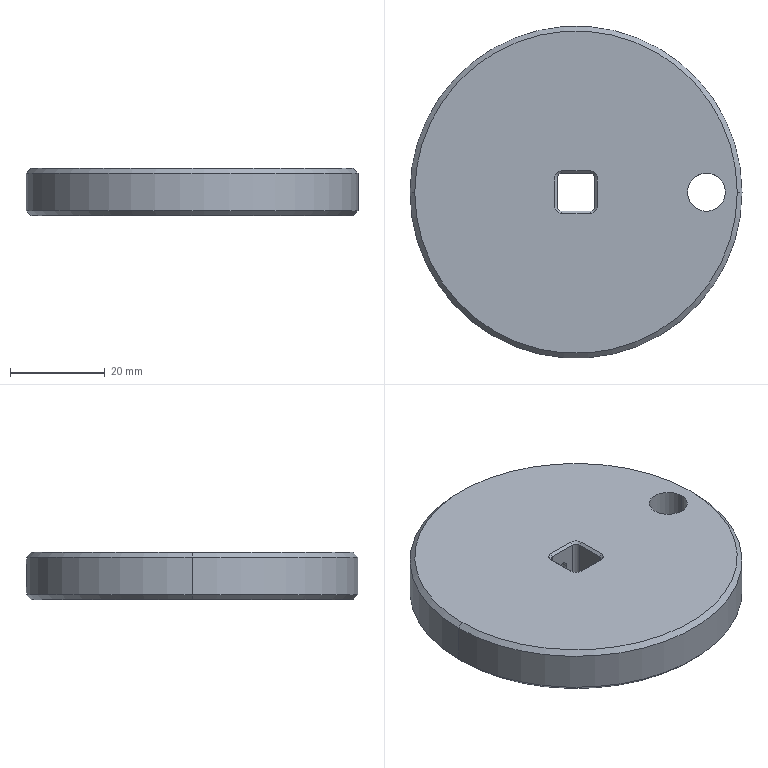Part | SolidWorks | features ICE 4, Chamfer 2, 3DProfileFeature 1, Cut 1, Extrusion 1, Fillet 1, HoleWzd 1 | 1 solid | 39 faces | box 70 x 70 x 10 mm | volume 36483 mm3 | plane 15 | cylinder 12 | cone 12 | commonest cylinder face diameters 2 x4 2.5 x2 6 x2 8 x2 70 x2
STEP:
#1=CARTESIAN_POINT('',(0.,4.,3.75));
#2=VERTEX_POINT('',#1);
#3=CARTESIAN_POINT('',(0.,4.,6.25));
#4=VERTEX_POINT('',#3);
#5=CARTESIAN_POINT('',(0.,4.,5.));
#6=DIRECTION('',(0.,1.,0.));
#7=DIRECTION('',(0.,0.,1.));
#8=AXIS2_PLACEMENT_3D('',#5,#6,#7);
#9=CIRCLE('',#8,1.25);
#10=EDGE_CURVE('',#2,#4,#9,.T.);
#11=ORIENTED_EDGE('',*,*,#10,.F.);
#12=CARTESIAN_POINT('',(0.,14.,3.75));
#13=VERTEX_POINT('',#12);
#14=CARTESIAN_POINT('',(0.,14.,3.75));
#15=DIRECTION('',(0.,1.,0.));
#16=VECTOR('',#15,1000.);
#17=LINE('',#14,#16);
#18=EDGE_CURVE('',#2,#13,#17,.T.);
#19=ORIENTED_EDGE('',*,*,#18,.T.);
#20=CARTESIAN_POINT('',(0.,14.,6.25));
#21=VERTEX_POINT('',#20);
#22=CARTESIAN_POINT('',(0.,14.,5.));
#23=DIRECTION('',(0.,1.,0.));
#24=DIRECTION('',(0.,0.,1.));
#25=AXIS2_PLACEMENT_3D('',#22,#23,#24);
#26=CIRCLE('',#25,1.25);
#27=EDGE_CURVE('',#13,#21,#26,.T.);
#28=ORIENTED_EDGE('',*,*,#27,.T.);
#29=CARTESIAN_POINT('',(0.,14.,6.25));
#30=DIRECTION('',(0.,1.,0.));
#31=VECTOR('',#30,1000.);
#32=LINE('',#29,#31);
#33=EDGE_CURVE('',#4,#21,#32,.T.);
#34=ORIENTED_EDGE('',*,*,#33,.F.);
#35=EDGE_LOOP('',(#11,#19,#28,#34));
#36=FACE_OUTER_BOUND('',#35,.T.);
#37=CARTESIAN_POINT('',(0.,14.,5.));
#38=DIRECTION('',(0.,1.,0.));
#39=DIRECTION('',(0.,0.,1.));
#40=AXIS2_PLACEMENT_3D('',#37,#38,#39);
#41=CYLINDRICAL_SURFACE('',#40,1.25);
#42=ADVANCED_FACE('',(#36),#41,.F.);
#43=CARTESIAN_POINT('',(0.,35.,2.));
#44=VERTEX_POINT('',#43);
#45=CARTESIAN_POINT('',(0.,35.,8.));
#46=VERTEX_POINT('',#45);
#47=CARTESIAN_POINT('',(0.,35.,2.));
#48=CARTESIAN_POINT('',(-0.1983,35.,2.));
#49=CARTESIAN_POINT('',(-0.3933,34.998,2.019));
#50=CARTESIAN_POINT('',(-0.7769,34.992,2.096));
#51=CARTESIAN_POINT('',(-0.9675,34.987,2.153));
#52=CARTESIAN_POINT('',(-1.331,34.975,2.304));
#53=CARTESIAN_POINT('',(-1.503,34.968,2.396));
#54=CARTESIAN_POINT('',(-1.829,34.953,2.614));
#55=CARTESIAN_POINT('',(-1.983,34.944,2.741));
#56=CARTESIAN_POINT('',(-2.26,34.927,3.017));
#57=CARTESIAN_POINT('',(-2.384,34.919,3.168));
#58=CARTESIAN_POINT('',(-2.603,34.903,3.496));
#59=CARTESIAN_POINT('',(-2.697,34.896,3.671));
#60=CARTESIAN_POINT('',(-2.846,34.884,4.032));
#61=CARTESIAN_POINT('',(-2.904,34.879,4.221));
#62=CARTESIAN_POINT('',(-2.981,34.873,4.608));
#63=CARTESIAN_POINT('',(-3.,34.871,4.803));
#64=CARTESIAN_POINT('',(-3.,34.871,5.195));
#65=CARTESIAN_POINT('',(-2.981,34.873,5.394));
#66=CARTESIAN_POINT('',(-2.904,34.879,5.778));
#67=CARTESIAN_POINT('',(-2.847,34.884,5.965));
#68=CARTESIAN_POINT('',(-2.697,34.896,6.329));
#69=CARTESIAN_POINT('',(-2.603,34.903,6.504));
#70=CARTESIAN_POINT('',(-2.386,34.919,6.829));
#71=CARTESIAN_POINT('',(-2.262,34.927,6.981));
#72=CARTESIAN_POINT('',(-1.982,34.944,7.261));
#73=CARTESIAN_POINT('',(-1.83,34.952,7.385));
#74=CARTESIAN_POINT('',(-1.505,34.968,7.602));
#75=CARTESIAN_POINT('',(-1.33,34.975,7.696));
#76=CARTESIAN_POINT('',(-0.9664,34.987,7.847));
#77=CARTESIAN_POINT('',(-0.7794,34.992,7.904));
#78=CARTESIAN_POINT('',(-0.3948,34.998,7.98));
#79=CARTESIAN_POINT('',(-0.1958,35.,8.));
#80=CARTESIAN_POINT('',(0.,35.,8.));
#81=B_SPLINE_CURVE_WITH_KNOTS('',3,(#47,#48,#49,#50,#51,#52,#53,#54,#55,#56,#57,#58,#59,#60,#61,#62,#63,#64,#65,#66,#67,#68,#69,#70,#71,#72,#73,#74,#75,#76,#77,#78,#79,#80),.UNSPECIFIED.,.F.,.F.,(4,2,2,2,2,2,2,2,2,2,2,2,2,2,2,2,4),(0.,0.0005865,0.001173,0.001759,0.002346,0.002932,0.003519,0.004105,0.004692,0.005278,0.005865,0.006451,0.007038,0.007624,0.008211,0.008797,0.009384),.UNSPECIFIED.);
#82=EDGE_CURVE('',#44,#46,#81,.T.);
#83=ORIENTED_EDGE('',*,*,#82,.T.);
#84=CARTESIAN_POINT('',(0.,14.,8.));
#85=VERTEX_POINT('',#84);
#86=CARTESIAN_POINT('',(0.,35.027,8.));
#87=DIRECTION('',(0.,-1.,0.));
#88=VECTOR('',#87,1000.);
#89=LINE('',#86,#88);
#90=EDGE_CURVE('',#46,#85,#89,.T.);
#91=ORIENTED_EDGE('',*,*,#90,.T.);
#92=CARTESIAN_POINT('',(0.,14.,2.));
#93=VERTEX_POINT('',#92);
#94=CARTESIAN_POINT('',(0.,14.,5.));
#95=DIRECTION('',(0.,1.,0.));
#96=DIRECTION('',(0.,0.,1.));
#97=AXIS2_PLACEMENT_3D('',#94,#95,#96);
#98=CIRCLE('',#97,3.);
#99=EDGE_CURVE('',#93,#85,#98,.T.);
#100=ORIENTED_EDGE('',*,*,#99,.F.);
#101=CARTESIAN_POINT('',(0.,35.027,2.));
#102=DIRECTION('',(0.,-1.,0.));
#103=VECTOR('',#102,1000.);
#104=LINE('',#101,#103);
#105=EDGE_CURVE('',#44,#93,#104,.T.);
#106=ORIENTED_EDGE('',*,*,#105,.F.);
#107=EDGE_LOOP('',(#83,#91,#100,#106));
#108=FACE_OUTER_BOUND('',#107,.T.);
#109=CARTESIAN_POINT('',(0.,35.027,5.));
#110=DIRECTION('',(0.,-1.,0.));
#111=DIRECTION('',(0.,0.,-1.));
#112=AXIS2_PLACEMENT_3D('',#109,#110,#111);
#113=CYLINDRICAL_SURFACE('',#112,3.);
#114=ADVANCED_FACE('',(#108),#113,.F.);
#115=CARTESIAN_POINT('',(23.5,0.,0.));
#116=VERTEX_POINT('',#115);
#117=CARTESIAN_POINT('',(31.5,0.,0.));
#118=VERTEX_POINT('',#117);
#119=CARTESIAN_POINT('',(27.5,0.,0.));
#120=DIRECTION('',(0.,0.,1.));
#121=DIRECTION('',(1.,0.,0.));
#122=AXIS2_PLACEMENT_3D('',#119,#120,#121);
#123=CIRCLE('',#122,4.);
#124=EDGE_CURVE('',#116,#118,#123,.T.);
#125=ORIENTED_EDGE('',*,*,#124,.F.);
#126=CARTESIAN_POINT('',(23.5,0.,10.));
#127=VERTEX_POINT('',#126);
#128=CARTESIAN_POINT('',(23.5,0.,-19.));
#129=DIRECTION('',(0.,0.,1.));
#130=VECTOR('',#129,1000.);
#131=LINE('',#128,#130);
#132=EDGE_CURVE('',#116,#127,#131,.T.);
#133=ORIENTED_EDGE('',*,*,#132,.T.);
#134=CARTESIAN_POINT('',(31.5,0.,10.));
#135=VERTEX_POINT('',#134);
#136=CARTESIAN_POINT('',(27.5,0.,10.));
#137=DIRECTION('',(0.,0.,1.));
#138=DIRECTION('',(1.,0.,0.));
#139=AXIS2_PLACEMENT_3D('',#136,#137,#138);
#140=CIRCLE('',#139,4.);
#141=EDGE_CURVE('',#127,#135,#140,.T.);
#142=ORIENTED_EDGE('',*,*,#141,.T.);
#143=CARTESIAN_POINT('',(31.5,0.,-19.));
#144=DIRECTION('',(0.,0.,1.));
#145=VECTOR('',#144,1000.);
#146=LINE('',#143,#145);
#147=EDGE_CURVE('',#118,#135,#146,.T.);
#148=ORIENTED_EDGE('',*,*,#147,.F.);
#149=EDGE_LOOP('',(#125,#133,#142,#148));
#150=FACE_OUTER_BOUND('',#149,.T.);
#151=CARTESIAN_POINT('',(27.5,0.,-19.));
#152=DIRECTION('',(0.,0.,1.));
#153=DIRECTION('',(1.,0.,0.));
#154=AXIS2_PLACEMENT_3D('',#151,#152,#153);
#155=CYLINDRICAL_SURFACE('',#154,4.);
#156=ADVANCED_FACE('',(#150),#155,.F.);
#157=CARTESIAN_POINT('',(34.,0.,10.));
#158=VERTEX_POINT('',#157);
#159=CARTESIAN_POINT('',(-34.,0.,10.));
#160=VERTEX_POINT('',#159);
#161=CARTESIAN_POINT('',(0.,0.,10.));
#162=DIRECTION('',(0.,0.,1.));
#163=DIRECTION('',(1.,0.,0.));
#164=AXIS2_PLACEMENT_3D('',#161,#162,#163);
#165=CIRCLE('',#164,34.);
#166=EDGE_CURVE('',#158,#160,#165,.T.);
#167=ORIENTED_EDGE('',*,*,#166,.F.);
#168=CARTESIAN_POINT('',(35.,0.,9.));
#169=VERTEX_POINT('',#168);
#170=CARTESIAN_POINT('',(34.,0.,10.));
#171=DIRECTION('',(0.7071,0.,-0.7071));
#172=VECTOR('',#171,1000.);
#173=LINE('',#170,#172);
#174=EDGE_CURVE('',#158,#169,#173,.T.);
#175=ORIENTED_EDGE('',*,*,#174,.T.);
#176=CARTESIAN_POINT('',(-35.,0.,9.));
#177=VERTEX_POINT('',#176);
#178=CARTESIAN_POINT('',(0.,0.,9.));
#179=DIRECTION('',(0.,0.,-1.));
#180=DIRECTION('',(1.,0.,0.));
#181=AXIS2_PLACEMENT_3D('',#178,#179,#180);
#182=CIRCLE('',#181,35.);
#183=EDGE_CURVE('',#177,#169,#182,.T.);
#184=ORIENTED_EDGE('',*,*,#183,.F.);
#185=CARTESIAN_POINT('',(-34.,0.,10.));
#186=DIRECTION('',(-0.7071,0.,-0.7071));
#187=VECTOR('',#186,1000.);
#188=LINE('',#185,#187);
#189=EDGE_CURVE('',#160,#177,#188,.T.);
#190=ORIENTED_EDGE('',*,*,#189,.F.);
#191=EDGE_LOOP('',(#167,#175,#184,#190));
#192=FACE_OUTER_BOUND('',#191,.T.);
#193=CARTESIAN_POINT('',(0.,0.,10.));
#194=DIRECTION('',(0.,0.,-1.));
#195=DIRECTION('',(-1.,0.,0.));
#196=AXIS2_PLACEMENT_3D('',#193,#194,#195);
#197=CONICAL_SURFACE('',#196,34.,0.7854);
#198=ADVANCED_FACE('',(#192),#197,.T.);
#199=CARTESIAN_POINT('',(-34.,0.,0.));
#200=VERTEX_POINT('',#199);
#201=CARTESIAN_POINT('',(34.,0.,0.));
#202=VERTEX_POINT('',#201);
#203=CARTESIAN_POINT('',(0.,0.,0.));
#204=DIRECTION('',(0.,0.,-1.));
#205=DIRECTION('',(1.,0.,0.));
#206=AXIS2_PLACEMENT_3D('',#203,#204,#205);
#207=CIRCLE('',#206,34.);
#208=EDGE_CURVE('',#200,#202,#207,.T.);
#209=ORIENTED_EDGE('',*,*,#208,.F.);
#210=CARTESIAN_POINT('',(-35.,0.,1.));
#211=VERTEX_POINT('',#210);
#212=CARTESIAN_POINT('',(-35.,0.,1.));
#213=DIRECTION('',(-0.7071,0.,0.7071));
#214=VECTOR('',#213,1000.);
#215=LINE('',#212,#214);
#216=EDGE_CURVE('',#200,#211,#215,.T.);
#217=ORIENTED_EDGE('',*,*,#216,.T.);
#218=CARTESIAN_POINT('',(35.,0.,1.));
#219=VERTEX_POINT('',#218);
#220=CARTESIAN_POINT('',(0.,0.,1.));
#221=DIRECTION('',(0.,0.,1.));
#222=DIRECTION('',(1.,0.,0.));
#223=AXIS2_PLACEMENT_3D('',#220,#221,#222);
#224=CIRCLE('',#223,35.);
#225=EDGE_CURVE('',#219,#211,#224,.T.);
#226=ORIENTED_EDGE('',*,*,#225,.F.);
#227=CARTESIAN_POINT('',(35.,0.,1.));
#228=DIRECTION('',(0.7071,0.,0.7071));
#229=VECTOR('',#228,1000.);
#230=LINE('',#227,#229);
#231=EDGE_CURVE('',#202,#219,#230,.T.);
#232=ORIENTED_EDGE('',*,*,#231,.F.);
#233=EDGE_LOOP('',(#209,#217,#226,#232));
#234=FACE_OUTER_BOUND('',#233,.T.);
#235=CARTESIAN_POINT('',(0.,0.,1.));
#236=DIRECTION('',(0.,0.,1.));
#237=DIRECTION('',(1.,0.,0.));
#238=AXIS2_PLACEMENT_3D('',#235,#236,#237);
#239=CONICAL_SURFACE('',#238,35.,0.7854);
#240=ADVANCED_FACE('',(#234),#239,.T.);
#241=ORIENTED_EDGE('',*,*,#82,.F.);
#242=CARTESIAN_POINT('',(0.,35.,8.));
#243=CARTESIAN_POINT('',(0.1958,35.,8.));
#244=CARTESIAN_POINT('',(0.3904,34.998,7.981));
#245=CARTESIAN_POINT('',(0.7774,34.992,7.904));
#246=CARTESIAN_POINT('',(0.9669,34.987,7.847));
#247=CARTESIAN_POINT('',(1.328,34.975,7.697));
#248=CARTESIAN_POINT('',(1.502,34.968,7.604));
#249=CARTESIAN_POINT('',(1.83,34.952,7.385));
#250=CARTESIAN_POINT('',(1.981,34.944,7.261));
#251=CARTESIAN_POINT('',(2.258,34.927,6.985));
#252=CARTESIAN_POINT('',(2.385,34.919,6.83));
#253=CARTESIAN_POINT('',(2.603,34.903,6.504));
#254=CARTESIAN_POINT('',(2.695,34.896,6.332));
#255=CARTESIAN_POINT('',(2.846,34.884,5.969));
#256=CARTESIAN_POINT('',(2.904,34.879,5.779));
#257=CARTESIAN_POINT('',(2.98,34.873,5.395));
#258=CARTESIAN_POINT('',(3.,34.871,5.2));
#259=CARTESIAN_POINT('',(3.,34.871,4.804));
#260=CARTESIAN_POINT('',(2.981,34.873,4.609));
#261=CARTESIAN_POINT('',(2.905,34.879,4.225));
#262=CARTESIAN_POINT('',(2.847,34.884,4.035));
#263=CARTESIAN_POINT('',(2.697,34.896,3.671));
#264=CARTESIAN_POINT('',(2.605,34.903,3.499));
#265=CARTESIAN_POINT('',(2.388,34.919,3.173));
#266=CARTESIAN_POINT('',(2.261,34.927,3.019));
#267=CARTESIAN_POINT('',(1.985,34.944,2.742));
#268=CARTESIAN_POINT('',(1.834,34.952,2.618));
#269=CARTESIAN_POINT('',(1.506,34.968,2.398));
#270=CARTESIAN_POINT('',(1.332,34.975,2.305));
#271=CARTESIAN_POINT('',(0.7905,34.993,2.08));
#272=CARTESIAN_POINT('',(0.3965,35.,2.));
#273=CARTESIAN_POINT('',(0.,35.,2.));
#274=B_SPLINE_CURVE_WITH_KNOTS('',3,(#242,#243,#244,#245,#246,#247,#248,#249,#250,#251,#252,#253,#254,#255,#256,#257,#258,#259,#260,#261,#262,#263,#264,#265,#266,#267,#268,#269,#270,#271,#272,#273),.UNSPECIFIED.,.F.,.F.,(4,2,2,2,2,2,2,2,2,2,2,2,2,2,2,4),(0.009384,0.00997,0.01056,0.01114,0.01173,0.01232,0.0129,0.01349,0.01407,0.01466,0.01525,0.01583,0.01642,0.01701,0.01759,0.01877),.UNSPECIFIED.);
#275=EDGE_CURVE('',#46,#44,#274,.T.);
#276=ORIENTED_EDGE('',*,*,#275,.F.);
#277=EDGE_LOOP('',(#241,#276));
#278=FACE_BOUND('',#277,.T.);
#279=ORIENTED_EDGE('',*,*,#183,.T.);
#280=CARTESIAN_POINT('',(35.,0.,10.));
#281=DIRECTION('',(0.,0.,-1.));
#282=VECTOR('',#281,1000.);
#283=LINE('',#280,#282);
#284=EDGE_CURVE('',#169,#219,#283,.T.);
#285=ORIENTED_EDGE('',*,*,#284,.T.);
#286=ORIENTED_EDGE('',*,*,#225,.T.);
#287=CARTESIAN_POINT('',(-35.,0.,10.));
#288=DIRECTION('',(0.,0.,-1.));
#289=VECTOR('',#288,1000.);
#290=LINE('',#287,#289);
#291=EDGE_CURVE('',#177,#211,#290,.T.);
#292=ORIENTED_EDGE('',*,*,#291,.F.);
#293=EDGE_LOOP('',(#279,#285,#286,#292));
#294=FACE_OUTER_BOUND('',#293,.T.);
#295=CARTESIAN_POINT('',(0.,0.,10.));
#296=DIRECTION('',(0.,0.,-1.));
#297=DIRECTION('',(-1.,0.,0.));
#298=AXIS2_PLACEMENT_3D('',#295,#296,#297);
#299=CYLINDRICAL_SURFACE('',#298,35.);
#300=ADVANCED_FACE('',(#278,#294),#299,.T.);
#301=ORIENTED_EDGE('',*,*,#284,.F.);
#302=CARTESIAN_POINT('',(0.,0.,9.));
#303=DIRECTION('',(0.,0.,-1.));
#304=DIRECTION('',(1.,0.,0.));
#305=AXIS2_PLACEMENT_3D('',#302,#303,#304);
#306=CIRCLE('',#305,35.);
#307=EDGE_CURVE('',#169,#177,#306,.T.);
#308=ORIENTED_EDGE('',*,*,#307,.T.);
#309=ORIENTED_EDGE('',*,*,#291,.T.);
#310=CARTESIAN_POINT('',(0.,0.,1.));
#311=DIRECTION('',(0.,0.,1.));
#312=DIRECTION('',(1.,0.,0.));
#313=AXIS2_PLACEMENT_3D('',#310,#311,#312);
#314=CIRCLE('',#313,35.);
#315=EDGE_CURVE('',#211,#219,#314,.T.);
#316=ORIENTED_EDGE('',*,*,#315,.T.);
#317=EDGE_LOOP('',(#301,#308,#309,#316));
#318=FACE_OUTER_BOUND('',#317,.T.);
#319=CARTESIAN_POINT('',(0.,0.,10.));
#320=DIRECTION('',(0.,0.,-1.));
#321=DIRECTION('',(-1.,0.,0.));
#322=AXIS2_PLACEMENT_3D('',#319,#320,#321);
#323=CYLINDRICAL_SURFACE('',#322,35.);
#324=ADVANCED_FACE('',(#318),#323,.T.);
#325=CARTESIAN_POINT('',(3.,4.5,10.));
#326=VERTEX_POINT('',#325);
#327=CARTESIAN_POINT('',(4.5,3.,10.));
#328=VERTEX_POINT('',#327);
#329=CARTESIAN_POINT('',(3.,3.,10.));
#330=DIRECTION('',(0.,0.,-1.));
#331=DIRECTION('',(1.,0.,0.));
#332=AXIS2_PLACEMENT_3D('',#329,#330,#331);
#333=CIRCLE('',#332,1.5);
#334=EDGE_CURVE('',#326,#328,#333,.T.);
#335=ORIENTED_EDGE('',*,*,#334,.T.);
#336=CARTESIAN_POINT('',(4.5,-3.,10.));
#337=VERTEX_POINT('',#336);
#338=CARTESIAN_POINT('',(4.5,-3.,10.));
#339=DIRECTION('',(0.,-1.,0.));
#340=VECTOR('',#339,1000.);
#341=LINE('',#338,#340);
#342=EDGE_CURVE('',#328,#337,#341,.T.);
#343=ORIENTED_EDGE('',*,*,#342,.T.);
#344=CARTESIAN_POINT('',(3.,-4.5,10.));
#345=VERTEX_POINT('',#344);
#346=CARTESIAN_POINT('',(3.,-3.,10.));
#347=DIRECTION('',(0.,0.,-1.));
#348=DIRECTION('',(1.,0.,0.));
#349=AXIS2_PLACEMENT_3D('',#346,#347,#348);
#350=CIRCLE('',#349,1.5);
#351=EDGE_CURVE('',#337,#345,#350,.T.);
#352=ORIENTED_EDGE('',*,*,#351,.T.);
#353=CARTESIAN_POINT('',(-3.,-4.5,10.));
#354=VERTEX_POINT('',#353);
#355=CARTESIAN_POINT('',(-3.,-4.5,10.));
#356=DIRECTION('',(-1.,0.,0.));
#357=VECTOR('',#356,1000.);
#358=LINE('',#355,#357);
#359=EDGE_CURVE('',#345,#354,#358,.T.);
#360=ORIENTED_EDGE('',*,*,#359,.T.);
#361=CARTESIAN_POINT('',(-4.5,-3.,10.));
#362=VERTEX_POINT('',#361);
#363=CARTESIAN_POINT('',(-3.,-3.,10.));
#364=DIRECTION('',(0.,0.,-1.));
#365=DIRECTION('',(1.,0.,0.));
#366=AXIS2_PLACEMENT_3D('',#363,#364,#365);
#367=CIRCLE('',#366,1.5);
#368=EDGE_CURVE('',#354,#362,#367,.T.);
#369=ORIENTED_EDGE('',*,*,#368,.T.);
#370=CARTESIAN_POINT('',(-4.5,3.,10.));
#371=VERTEX_POINT('',#370);
#372=CARTESIAN_POINT('',(-4.5,3.,10.));
#373=DIRECTION('',(0.,1.,0.));
#374=VECTOR('',#373,1000.);
#375=LINE('',#372,#374);
#376=EDGE_CURVE('',#362,#371,#375,.T.);
#377=ORIENTED_EDGE('',*,*,#376,.T.);
#378=CARTESIAN_POINT('',(-3.,4.5,10.));
#379=VERTEX_POINT('',#378);
#380=CARTESIAN_POINT('',(-3.,3.,10.));
#381=DIRECTION('',(0.,0.,-1.));
#382=DIRECTION('',(1.,0.,0.));
#383=AXIS2_PLACEMENT_3D('',#380,#381,#382);
#384=CIRCLE('',#383,1.5);
#385=EDGE_CURVE('',#371,#379,#384,.T.);
#386=ORIENTED_EDGE('',*,*,#385,.T.);
#387=CARTESIAN_POINT('',(3.,4.5,10.));
#388=DIRECTION('',(1.,0.,0.));
#389=VECTOR('',#388,1000.);
#390=LINE('',#387,#389);
#391=EDGE_CURVE('',#379,#326,#390,.T.);
#392=ORIENTED_EDGE('',*,*,#391,.T.);
#393=EDGE_LOOP('',(#335,#343,#352,#360,#369,#377,#386,#392));
#394=FACE_BOUND('',#393,.T.);
#395=CARTESIAN_POINT('',(27.5,0.,10.));
#396=DIRECTION('',(0.,0.,1.));
#397=DIRECTION('',(1.,0.,0.));
#398=AXIS2_PLACEMENT_3D('',#395,#396,#397);
#399=CIRCLE('',#398,4.);
#400=EDGE_CURVE('',#135,#127,#399,.T.);
#401=ORIENTED_EDGE('',*,*,#400,.F.);
#402=ORIENTED_EDGE('',*,*,#141,.F.);
#403=EDGE_LOOP('',(#401,#402));
#404=FACE_BOUND('',#403,.T.);
#405=CARTESIAN_POINT('',(0.,0.,10.));
#406=DIRECTION('',(0.,0.,1.));
#407=DIRECTION('',(1.,0.,0.));
#408=AXIS2_PLACEMENT_3D('',#405,#406,#407);
#409=CIRCLE('',#408,34.);
#410=EDGE_CURVE('',#160,#158,#409,.T.);
#411=ORIENTED_EDGE('',*,*,#410,.T.);
#412=ORIENTED_EDGE('',*,*,#166,.T.);
#413=EDGE_LOOP('',(#411,#412));
#414=FACE_OUTER_BOUND('',#413,.T.);
#415=CARTESIAN_POINT('',(0.,0.,10.));
#416=DIRECTION('',(0.,0.,1.));
#417=DIRECTION('',(1.,0.,0.));
#418=AXIS2_PLACEMENT_3D('',#415,#416,#417);
#419=PLANE('',#418);
#420=ADVANCED_FACE('',(#394,#404,#414),#419,.T.);
#421=CARTESIAN_POINT('',(-4.5,-3.,0.));
#422=VERTEX_POINT('',#421);
#423=CARTESIAN_POINT('',(-3.,-4.5,0.));
#424=VERTEX_POINT('',#423);
#425=CARTESIAN_POINT('',(-3.,-3.,0.));
#426=DIRECTION('',(0.,0.,1.));
#427=DIRECTION('',(1.,0.,0.));
#428=AXIS2_PLACEMENT_3D('',#425,#426,#427);
#429=CIRCLE('',#428,1.5);
#430=EDGE_CURVE('',#422,#424,#429,.T.);
#431=ORIENTED_EDGE('',*,*,#430,.T.);
#432=CARTESIAN_POINT('',(3.,-4.5,0.));
#433=VERTEX_POINT('',#432);
#434=CARTESIAN_POINT('',(0.,-4.5,0.));
#435=DIRECTION('',(1.,0.,0.));
#436=VECTOR('',#435,1000.);
#437=LINE('',#434,#436);
#438=EDGE_CURVE('',#424,#433,#437,.T.);
#439=ORIENTED_EDGE('',*,*,#438,.T.);
#440=CARTESIAN_POINT('',(4.5,-3.,0.));
#441=VERTEX_POINT('',#440);
#442=CARTESIAN_POINT('',(3.,-3.,0.));
#443=DIRECTION('',(0.,0.,1.));
#444=DIRECTION('',(1.,0.,0.));
#445=AXIS2_PLACEMENT_3D('',#442,#443,#444);
#446=CIRCLE('',#445,1.5);
#447=EDGE_CURVE('',#433,#441,#446,.T.);
#448=ORIENTED_EDGE('',*,*,#447,.T.);
#449=CARTESIAN_POINT('',(4.5,3.,0.));
#450=VERTEX_POINT('',#449);
#451=CARTESIAN_POINT('',(4.5,0.,0.));
#452=DIRECTION('',(0.,1.,0.));
#453=VECTOR('',#452,1000.);
#454=LINE('',#451,#453);
#455=EDGE_CURVE('',#441,#450,#454,.T.);
#456=ORIENTED_EDGE('',*,*,#455,.T.);
#457=CARTESIAN_POINT('',(3.,4.5,0.));
#458=VERTEX_POINT('',#457);
#459=CARTESIAN_POINT('',(3.,3.,0.));
#460=DIRECTION('',(0.,0.,1.));
#461=DIRECTION('',(1.,0.,0.));
#462=AXIS2_PLACEMENT_3D('',#459,#460,#461);
#463=CIRCLE('',#462,1.5);
#464=EDGE_CURVE('',#450,#458,#463,.T.);
#465=ORIENTED_EDGE('',*,*,#464,.T.);
#466=CARTESIAN_POINT('',(-3.,4.5,0.));
#467=VERTEX_POINT('',#466);
#468=CARTESIAN_POINT('',(0.,4.5,0.));
#469=DIRECTION('',(-1.,0.,0.));
#470=VECTOR('',#469,1000.);
#471=LINE('',#468,#470);
#472=EDGE_CURVE('',#458,#467,#471,.T.);
#473=ORIENTED_EDGE('',*,*,#472,.T.);
#474=CARTESIAN_POINT('',(-4.5,3.,0.));
#475=VERTEX_POINT('',#474);
#476=CARTESIAN_POINT('',(-3.,3.,0.));
#477=DIRECTION('',(0.,0.,1.));
#478=DIRECTION('',(1.,0.,0.));
#479=AXIS2_PLACEMENT_3D('',#476,#477,#478);
#480=CIRCLE('',#479,1.5);
#481=EDGE_CURVE('',#467,#475,#480,.T.);
#482=ORIENTED_EDGE('',*,*,#481,.T.);
#483=CARTESIAN_POINT('',(-4.5,0.,0.));
#484=DIRECTION('',(0.,-1.,0.));
#485=VECTOR('',#484,1000.);
#486=LINE('',#483,#485);
#487=EDGE_CURVE('',#475,#422,#486,.T.);
#488=ORIENTED_EDGE('',*,*,#487,.T.);
#489=EDGE_LOOP('',(#431,#439,#448,#456,#465,#473,#482,#488));
#490=FACE_BOUND('',#489,.T.);
#491=CARTESIAN_POINT('',(27.5,0.,0.));
#492=DIRECTION('',(0.,0.,1.));
#493=DIRECTION('',(1.,0.,0.));
#494=AXIS2_PLACEMENT_3D('',#491,#492,#493);
#495=CIRCLE('',#494,4.);
#496=EDGE_CURVE('',#118,#116,#495,.T.);
#497=ORIENTED_EDGE('',*,*,#496,.T.);
#498=ORIENTED_EDGE('',*,*,#124,.T.);
#499=EDGE_LOOP('',(#497,#498));
#500=FACE_BOUND('',#499,.T.);
#501=CARTESIAN_POINT('',(0.,0.,0.));
#502=DIRECTION('',(0.,0.,-1.));
#503=DIRECTION('',(1.,0.,0.));
#504=AXIS2_PLACEMENT_3D('',#501,#502,#503);
#505=CIRCLE('',#504,34.);
#506=EDGE_CURVE('',#202,#200,#505,.T.);
#507=ORIENTED_EDGE('',*,*,#506,.T.);
#508=ORIENTED_EDGE('',*,*,#208,.T.);
#509=EDGE_LOOP('',(#507,#508));
#510=FACE_OUTER_BOUND('',#509,.T.);
#511=CARTESIAN_POINT('',(0.,0.,0.));
#512=DIRECTION('',(0.,0.,1.));
#513=DIRECTION('',(1.,0.,0.));
#514=AXIS2_PLACEMENT_3D('',#511,#512,#513);
#515=PLANE('',#514);
#516=ADVANCED_FACE('',(#490,#500,#510),#515,.F.);
#517=ORIENTED_EDGE('',*,*,#216,.F.);
#518=ORIENTED_EDGE('',*,*,#506,.F.);
#519=ORIENTED_EDGE('',*,*,#231,.T.);
#520=ORIENTED_EDGE('',*,*,#315,.F.);
#521=EDGE_LOOP('',(#517,#518,#519,#520));
#522=FACE_OUTER_BOUND('',#521,.T.);
#523=CARTESIAN_POINT('',(0.,0.,1.));
#524=DIRECTION('',(0.,0.,1.));
#525=DIRECTION('',(1.,0.,0.));
#526=AXIS2_PLACEMENT_3D('',#523,#524,#525);
#527=CONICAL_SURFACE('',#526,35.,0.7854);
#528=ADVANCED_FACE('',(#522),#527,.T.);
#529=ORIENTED_EDGE('',*,*,#174,.F.);
#530=ORIENTED_EDGE('',*,*,#410,.F.);
#531=ORIENTED_EDGE('',*,*,#189,.T.);
#532=ORIENTED_EDGE('',*,*,#307,.F.);
#533=EDGE_LOOP('',(#529,#530,#531,#532));
#534=FACE_OUTER_BOUND('',#533,.T.);
#535=CARTESIAN_POINT('',(0.,0.,10.));
#536=DIRECTION('',(0.,0.,-1.));
#537=DIRECTION('',(-1.,0.,0.));
#538=AXIS2_PLACEMENT_3D('',#535,#536,#537);
#539=CONICAL_SURFACE('',#538,34.,0.7854);
#540=ADVANCED_FACE('',(#534),#539,.T.);
#541=ORIENTED_EDGE('',*,*,#132,.F.);
#542=ORIENTED_EDGE('',*,*,#496,.F.);
#543=ORIENTED_EDGE('',*,*,#147,.T.);
#544=ORIENTED_EDGE('',*,*,#400,.T.);
#545=EDGE_LOOP('',(#541,#542,#543,#544));
#546=FACE_OUTER_BOUND('',#545,.T.);
#547=CARTESIAN_POINT('',(27.5,0.,-19.));
#548=DIRECTION('',(0.,0.,1.));
#549=DIRECTION('',(1.,0.,0.));
#550=AXIS2_PLACEMENT_3D('',#547,#548,#549);
#551=CYLINDRICAL_SURFACE('',#550,4.);
#552=ADVANCED_FACE('',(#546),#551,.F.);
#553=CARTESIAN_POINT('',(4.,3.,9.5));
#554=VERTEX_POINT('',#553);
#555=CARTESIAN_POINT('',(4.,3.,0.5));
#556=VERTEX_POINT('',#555);
#557=CARTESIAN_POINT('',(4.,3.,0.));
#558=DIRECTION('',(0.,0.,-1.));
#559=VECTOR('',#558,1000.);
#560=LINE('',#557,#559);
#561=EDGE_CURVE('',#554,#556,#560,.T.);
#562=ORIENTED_EDGE('',*,*,#561,.T.);
#563=CARTESIAN_POINT('',(4.,-3.,0.5));
#564=VERTEX_POINT('',#563);
#565=CARTESIAN_POINT('',(4.,4.,0.5));
#566=DIRECTION('',(0.,-1.,0.));
#567=VECTOR('',#566,1000.);
#568=LINE('',#565,#567);
#569=EDGE_CURVE('',#556,#564,#568,.T.);
#570=ORIENTED_EDGE('',*,*,#569,.T.);
#571=CARTESIAN_POINT('',(4.,-3.,9.5));
#572=VERTEX_POINT('',#571);
#573=CARTESIAN_POINT('',(4.,-3.,10.));
#574=DIRECTION('',(0.,0.,1.));
#575=VECTOR('',#574,1000.);
#576=LINE('',#573,#575);
#577=EDGE_CURVE('',#564,#572,#576,.T.);
#578=ORIENTED_EDGE('',*,*,#577,.T.);
#579=CARTESIAN_POINT('',(4.,3.,9.5));
#580=DIRECTION('',(0.,1.,0.));
#581=VECTOR('',#580,1000.);
#582=LINE('',#579,#581);
#583=EDGE_CURVE('',#572,#554,#582,.T.);
#584=ORIENTED_EDGE('',*,*,#583,.T.);
#585=EDGE_LOOP('',(#562,#570,#578,#584));
#586=FACE_OUTER_BOUND('',#585,.T.);
#587=CARTESIAN_POINT('',(4.,4.,0.));
#588=DIRECTION('',(1.,0.,0.));
#589=DIRECTION('',(0.,1.,0.));
#590=AXIS2_PLACEMENT_3D('',#587,#588,#589);
#591=PLANE('',#590);
#592=ADVANCED_FACE('',(#586),#591,.F.);
#593=CARTESIAN_POINT('',(3.,-4.,9.5));
#594=VERTEX_POINT('',#593);
#595=CARTESIAN_POINT('',(3.,-4.,0.5));
#596=VERTEX_POINT('',#595);
#597=CARTESIAN_POINT('',(3.,-4.,0.));
#598=DIRECTION('',(0.,0.,-1.));
#599=VECTOR('',#598,1000.);
#600=LINE('',#597,#599);
#601=EDGE_CURVE('',#594,#596,#600,.T.);
#602=ORIENTED_EDGE('',*,*,#601,.T.);
#603=CARTESIAN_POINT('',(-3.,-4.,0.5));
#604=VERTEX_POINT('',#603);
#605=CARTESIAN_POINT('',(-4.,-4.,0.5));
#606=DIRECTION('',(-1.,0.,0.));
#607=VECTOR('',#606,1000.);
#608=LINE('',#605,#607);
#609=EDGE_CURVE('',#596,#604,#608,.T.);
#610=ORIENTED_EDGE('',*,*,#609,.T.);
#611=CARTESIAN_POINT('',(-3.,-4.,9.5));
#612=VERTEX_POINT('',#611);
#613=CARTESIAN_POINT('',(-3.,-4.,10.));
#614=DIRECTION('',(0.,0.,1.));
#615=VECTOR('',#614,1000.);
#616=LINE('',#613,#615);
#617=EDGE_CURVE('',#604,#612,#616,.T.);
#618=ORIENTED_EDGE('',*,*,#617,.T.);
#619=CARTESIAN_POINT('',(3.,-4.,9.5));
#620=DIRECTION('',(1.,0.,0.));
#621=VECTOR('',#620,1000.);
#622=LINE('',#619,#621);
#623=EDGE_CURVE('',#612,#594,#622,.T.);
#624=ORIENTED_EDGE('',*,*,#623,.T.);
#625=EDGE_LOOP('',(#602,#610,#618,#624));
#626=FACE_OUTER_BOUND('',#625,.T.);
#627=CARTESIAN_POINT('',(-4.,-4.,0.));
#628=DIRECTION('',(0.,-1.,0.));
#629=DIRECTION('',(0.,0.,-1.));
#630=AXIS2_PLACEMENT_3D('',#627,#628,#629);
#631=PLANE('',#630);
#632=ADVANCED_FACE('',(#626),#631,.F.);
#633=CARTESIAN_POINT('',(-4.,-3.,9.5));
#634=VERTEX_POINT('',#633);
#635=CARTESIAN_POINT('',(-4.,-3.,0.5));
#636=VERTEX_POINT('',#635);
#637=CARTESIAN_POINT('',(-4.,-3.,0.));
#638=DIRECTION('',(0.,0.,-1.));
#639=VECTOR('',#638,1000.);
#640=LINE('',#637,#639);
#641=EDGE_CURVE('',#634,#636,#640,.T.);
#642=ORIENTED_EDGE('',*,*,#641,.T.);
#643=CARTESIAN_POINT('',(-4.,3.,0.5));
#644=VERTEX_POINT('',#643);
#645=CARTESIAN_POINT('',(-4.,4.,0.5));
#646=DIRECTION('',(0.,1.,0.));
#647=VECTOR('',#646,1000.);
#648=LINE('',#645,#647);
#649=EDGE_CURVE('',#636,#644,#648,.T.);
#650=ORIENTED_EDGE('',*,*,#649,.T.);
#651=CARTESIAN_POINT('',(-4.,3.,9.5));
#652=VERTEX_POINT('',#651);
#653=CARTESIAN_POINT('',(-4.,3.,10.));
#654=DIRECTION('',(0.,0.,1.));
#655=VECTOR('',#654,1000.);
#656=LINE('',#653,#655);
#657=EDGE_CURVE('',#644,#652,#656,.T.);
#658=ORIENTED_EDGE('',*,*,#657,.T.);
#659=CARTESIAN_POINT('',(-4.,-3.,9.5));
#660=DIRECTION('',(0.,-1.,0.));
#661=VECTOR('',#660,1000.);
#662=LINE('',#659,#661);
#663=EDGE_CURVE('',#652,#634,#662,.T.);
#664=ORIENTED_EDGE('',*,*,#663,.T.);
#665=EDGE_LOOP('',(#642,#650,#658,#664));
#666=FACE_OUTER_BOUND('',#665,.T.);
#667=CARTESIAN_POINT('',(-4.,4.,0.));
#668=DIRECTION('',(-1.,0.,0.));
#669=DIRECTION('',(0.,-1.,0.));
#670=AXIS2_PLACEMENT_3D('',#667,#668,#669);
#671=PLANE('',#670);
#672=ADVANCED_FACE('',(#666),#671,.F.);
#673=CARTESIAN_POINT('',(0.,4.,5.));
#674=DIRECTION('',(0.,1.,0.));
#675=DIRECTION('',(0.,0.,1.));
#676=AXIS2_PLACEMENT_3D('',#673,#674,#675);
#677=CIRCLE('',#676,1.25);
#678=EDGE_CURVE('',#4,#2,#677,.T.);
#679=ORIENTED_EDGE('',*,*,#678,.T.);
#680=ORIENTED_EDGE('',*,*,#10,.T.);
#681=EDGE_LOOP('',(#679,#680));
#682=FACE_BOUND('',#681,.T.);
#683=CARTESIAN_POINT('',(-3.,4.,9.5));
#684=VERTEX_POINT('',#683);
#685=CARTESIAN_POINT('',(-3.,4.,0.5));
#686=VERTEX_POINT('',#685);
#687=CARTESIAN_POINT('',(-3.,4.,0.));
#688=DIRECTION('',(0.,0.,-1.));
#689=VECTOR('',#688,1000.);
#690=LINE('',#687,#689);
#691=EDGE_CURVE('',#684,#686,#690,.T.);
#692=ORIENTED_EDGE('',*,*,#691,.T.);
#693=CARTESIAN_POINT('',(3.,4.,0.5));
#694=VERTEX_POINT('',#693);
#695=CARTESIAN_POINT('',(-4.,4.,0.5));
#696=DIRECTION('',(1.,0.,0.));
#697=VECTOR('',#696,1000.);
#698=LINE('',#695,#697);
#699=EDGE_CURVE('',#686,#694,#698,.T.);
#700=ORIENTED_EDGE('',*,*,#699,.T.);
#701=CARTESIAN_POINT('',(3.,4.,9.5));
#702=VERTEX_POINT('',#701);
#703=CARTESIAN_POINT('',(3.,4.,10.));
#704=DIRECTION('',(0.,0.,1.));
#705=VECTOR('',#704,1000.);
#706=LINE('',#703,#705);
#707=EDGE_CURVE('',#694,#702,#706,.T.);
#708=ORIENTED_EDGE('',*,*,#707,.T.);
#709=CARTESIAN_POINT('',(-3.,4.,9.5));
#710=DIRECTION('',(-1.,0.,0.));
#711=VECTOR('',#710,1000.);
#712=LINE('',#709,#711);
#713=EDGE_CURVE('',#702,#684,#712,.T.);
#714=ORIENTED_EDGE('',*,*,#713,.T.);
#715=EDGE_LOOP('',(#692,#700,#708,#714));
#716=FACE_OUTER_BOUND('',#715,.T.);
#717=CARTESIAN_POINT('',(-4.,4.,0.));
#718=DIRECTION('',(0.,1.,0.));
#719=DIRECTION('',(0.,0.,1.));
#720=AXIS2_PLACEMENT_3D('',#717,#718,#719);
#721=PLANE('',#720);
#722=ADVANCED_FACE('',(#682,#716),#721,.F.);
#723=ORIENTED_EDGE('',*,*,#617,.F.);
#724=CARTESIAN_POINT('',(-3.,-3.,0.5));
#725=DIRECTION('',(0.,0.,-1.));
#726=DIRECTION('',(1.,0.,0.));
#727=AXIS2_PLACEMENT_3D('',#724,#725,#726);
#728=CIRCLE('',#727,1.);
#729=EDGE_CURVE('',#604,#636,#728,.T.);
#730=ORIENTED_EDGE('',*,*,#729,.T.);
#731=ORIENTED_EDGE('',*,*,#641,.F.);
#732=CARTESIAN_POINT('',(-3.,-3.,9.5));
#733=DIRECTION('',(0.,0.,1.));
#734=DIRECTION('',(1.,0.,0.));
#735=AXIS2_PLACEMENT_3D('',#732,#733,#734);
#736=CIRCLE('',#735,1.);
#737=EDGE_CURVE('',#634,#612,#736,.T.);
#738=ORIENTED_EDGE('',*,*,#737,.T.);
#739=EDGE_LOOP('',(#723,#730,#731,#738));
#740=FACE_OUTER_BOUND('',#739,.T.);
#741=CARTESIAN_POINT('',(-3.,-3.,0.));
#742=DIRECTION('',(0.,0.,-1.));
#743=DIRECTION('',(-1.,0.,0.));
#744=AXIS2_PLACEMENT_3D('',#741,#742,#743);
#745=CYLINDRICAL_SURFACE('',#744,1.);
#746=ADVANCED_FACE('',(#740),#745,.F.);
#747=ORIENTED_EDGE('',*,*,#577,.F.);
#748=CARTESIAN_POINT('',(3.,-3.,0.5));
#749=DIRECTION('',(0.,0.,-1.));
#750=DIRECTION('',(1.,0.,0.));
#751=AXIS2_PLACEMENT_3D('',#748,#749,#750);
#752=CIRCLE('',#751,1.);
#753=EDGE_CURVE('',#564,#596,#752,.T.);
#754=ORIENTED_EDGE('',*,*,#753,.T.);
#755=ORIENTED_EDGE('',*,*,#601,.F.);
#756=CARTESIAN_POINT('',(3.,-3.,9.5));
#757=DIRECTION('',(0.,0.,1.));
#758=DIRECTION('',(1.,0.,0.));
#759=AXIS2_PLACEMENT_3D('',#756,#757,#758);
#760=CIRCLE('',#759,1.);
#761=EDGE_CURVE('',#594,#572,#760,.T.);
#762=ORIENTED_EDGE('',*,*,#761,.T.);
#763=EDGE_LOOP('',(#747,#754,#755,#762));
#764=FACE_OUTER_BOUND('',#763,.T.);
#765=CARTESIAN_POINT('',(3.,-3.,0.));
#766=DIRECTION('',(0.,0.,-1.));
#767=DIRECTION('',(-1.,0.,0.));
#768=AXIS2_PLACEMENT_3D('',#765,#766,#767);
#769=CYLINDRICAL_SURFACE('',#768,1.);
#770=ADVANCED_FACE('',(#764),#769,.F.);
#771=ORIENTED_EDGE('',*,*,#707,.F.);
#772=CARTESIAN_POINT('',(3.,3.,0.5));
#773=DIRECTION('',(0.,0.,-1.));
#774=DIRECTION('',(1.,0.,0.));
#775=AXIS2_PLACEMENT_3D('',#772,#773,#774);
#776=CIRCLE('',#775,1.);
#777=EDGE_CURVE('',#694,#556,#776,.T.);
#778=ORIENTED_EDGE('',*,*,#777,.T.);
#779=ORIENTED_EDGE('',*,*,#561,.F.);
#780=CARTESIAN_POINT('',(3.,3.,9.5));
#781=DIRECTION('',(0.,0.,1.));
#782=DIRECTION('',(1.,0.,0.));
#783=AXIS2_PLACEMENT_3D('',#780,#781,#782);
#784=CIRCLE('',#783,1.);
#785=EDGE_CURVE('',#554,#702,#784,.T.);
#786=ORIENTED_EDGE('',*,*,#785,.T.);
#787=EDGE_LOOP('',(#771,#778,#779,#786));
#788=FACE_OUTER_BOUND('',#787,.T.);
#789=CARTESIAN_POINT('',(3.,3.,0.));
#790=DIRECTION('',(0.,0.,-1.));
#791=DIRECTION('',(-1.,0.,0.));
#792=AXIS2_PLACEMENT_3D('',#789,#790,#791);
#793=CYLINDRICAL_SURFACE('',#792,1.);
#794=ADVANCED_FACE('',(#788),#793,.F.);
#795=ORIENTED_EDGE('',*,*,#657,.F.);
#796=CARTESIAN_POINT('',(-3.,3.,0.5));
#797=DIRECTION('',(0.,0.,-1.));
#798=DIRECTION('',(1.,0.,0.));
#799=AXIS2_PLACEMENT_3D('',#796,#797,#798);
#800=CIRCLE('',#799,1.);
#801=EDGE_CURVE('',#644,#686,#800,.T.);
#802=ORIENTED_EDGE('',*,*,#801,.T.);
#803=ORIENTED_EDGE('',*,*,#691,.F.);
#804=CARTESIAN_POINT('',(-3.,3.,9.5));
#805=DIRECTION('',(0.,0.,1.));
#806=DIRECTION('',(1.,0.,0.));
#807=AXIS2_PLACEMENT_3D('',#804,#805,#806);
#808=CIRCLE('',#807,1.);
#809=EDGE_CURVE('',#684,#652,#808,.T.);
#810=ORIENTED_EDGE('',*,*,#809,.T.);
#811=EDGE_LOOP('',(#795,#802,#803,#810));
#812=FACE_OUTER_BOUND('',#811,.T.);
#813=CARTESIAN_POINT('',(-3.,3.,0.));
#814=DIRECTION('',(0.,0.,-1.));
#815=DIRECTION('',(-1.,0.,0.));
#816=AXIS2_PLACEMENT_3D('',#813,#814,#815);
#817=CYLINDRICAL_SURFACE('',#816,1.);
#818=ADVANCED_FACE('',(#812),#817,.F.);
#819=ORIENTED_EDGE('',*,*,#90,.F.);
#820=ORIENTED_EDGE('',*,*,#275,.T.);
#821=ORIENTED_EDGE('',*,*,#105,.T.);
#822=CARTESIAN_POINT('',(0.,14.,5.));
#823=DIRECTION('',(0.,1.,0.));
#824=DIRECTION('',(0.,0.,1.));
#825=AXIS2_PLACEMENT_3D('',#822,#823,#824);
#826=CIRCLE('',#825,3.);
#827=EDGE_CURVE('',#85,#93,#826,.T.);
#828=ORIENTED_EDGE('',*,*,#827,.F.);
#829=EDGE_LOOP('',(#819,#820,#821,#828));
#830=FACE_OUTER_BOUND('',#829,.T.);
#831=CARTESIAN_POINT('',(0.,35.027,5.));
#832=DIRECTION('',(0.,-1.,0.));
#833=DIRECTION('',(0.,0.,-1.));
#834=AXIS2_PLACEMENT_3D('',#831,#832,#833);
#835=CYLINDRICAL_SURFACE('',#834,3.);
#836=ADVANCED_FACE('',(#830),#835,.F.);
#837=CARTESIAN_POINT('',(0.,14.,5.));
#838=DIRECTION('',(0.,1.,0.));
#839=DIRECTION('',(0.,0.,1.));
#840=AXIS2_PLACEMENT_3D('',#837,#838,#839);
#841=CIRCLE('',#840,1.25);
#842=EDGE_CURVE('',#21,#13,#841,.T.);
#843=ORIENTED_EDGE('',*,*,#842,.F.);
#844=ORIENTED_EDGE('',*,*,#27,.F.);
#845=EDGE_LOOP('',(#843,#844));
#846=FACE_BOUND('',#845,.T.);
#847=ORIENTED_EDGE('',*,*,#99,.T.);
#848=ORIENTED_EDGE('',*,*,#827,.T.);
#849=EDGE_LOOP('',(#847,#848));
#850=FACE_OUTER_BOUND('',#849,.T.);
#851=CARTESIAN_POINT('',(0.,14.,5.));
#852=DIRECTION('',(0.,1.,0.));
#853=DIRECTION('',(0.,0.,1.));
#854=AXIS2_PLACEMENT_3D('',#851,#852,#853);
#855=PLANE('',#854);
#856=ADVANCED_FACE('',(#846,#850),#855,.T.);
#857=ORIENTED_EDGE('',*,*,#18,.F.);
#858=ORIENTED_EDGE('',*,*,#678,.F.);
#859=ORIENTED_EDGE('',*,*,#33,.T.);
#860=ORIENTED_EDGE('',*,*,#842,.T.);
#861=EDGE_LOOP('',(#857,#858,#859,#860));
#862=FACE_OUTER_BOUND('',#861,.T.);
#863=CARTESIAN_POINT('',(0.,14.,5.));
#864=DIRECTION('',(0.,1.,0.));
#865=DIRECTION('',(0.,0.,1.));
#866=AXIS2_PLACEMENT_3D('',#863,#864,#865);
#867=CYLINDRICAL_SURFACE('',#866,1.25);
#868=ADVANCED_FACE('',(#862),#867,.F.);
#869=CARTESIAN_POINT('',(3.,4.,0.5));
#870=DIRECTION('',(0.,0.7071,-0.7071));
#871=VECTOR('',#870,1000.);
#872=LINE('',#869,#871);
#873=EDGE_CURVE('',#694,#458,#872,.T.);
#874=ORIENTED_EDGE('',*,*,#873,.F.);
#875=ORIENTED_EDGE('',*,*,#699,.F.);
#876=CARTESIAN_POINT('',(-3.,4.5,0.));
#877=DIRECTION('',(0.,-0.7071,0.7071));
#878=VECTOR('',#877,1000.);
#879=LINE('',#876,#878);
#880=EDGE_CURVE('',#467,#686,#879,.T.);
#881=ORIENTED_EDGE('',*,*,#880,.F.);
#882=ORIENTED_EDGE('',*,*,#472,.F.);
#883=EDGE_LOOP('',(#874,#875,#881,#882));
#884=FACE_OUTER_BOUND('',#883,.T.);
#885=CARTESIAN_POINT('',(0.,4.5,0.));
#886=DIRECTION('',(0.,0.7071,0.7071));
#887=DIRECTION('',(-1.,0.,0.));
#888=AXIS2_PLACEMENT_3D('',#885,#886,#887);
#889=PLANE('',#888);
#890=ADVANCED_FACE('',(#884),#889,.F.);
#891=ORIENTED_EDGE('',*,*,#880,.T.);
#892=ORIENTED_EDGE('',*,*,#801,.F.);
#893=CARTESIAN_POINT('',(-4.5,3.,0.));
#894=DIRECTION('',(0.7071,0.,0.7071));
#895=VECTOR('',#894,1000.);
#896=LINE('',#893,#895);
#897=EDGE_CURVE('',#475,#644,#896,.T.);
#898=ORIENTED_EDGE('',*,*,#897,.F.);
#899=ORIENTED_EDGE('',*,*,#481,.F.);
#900=EDGE_LOOP('',(#891,#892,#898,#899));
#901=FACE_OUTER_BOUND('',#900,.T.);
#902=CARTESIAN_POINT('',(-3.,3.,0.));
#903=DIRECTION('',(0.,0.,-1.));
#904=DIRECTION('',(-1.,0.,0.));
#905=AXIS2_PLACEMENT_3D('',#902,#903,#904);
#906=CONICAL_SURFACE('',#905,1.5,0.7854);
#907=ADVANCED_FACE('',(#901),#906,.F.);
#908=ORIENTED_EDGE('',*,*,#873,.T.);
#909=ORIENTED_EDGE('',*,*,#464,.F.);
#910=CARTESIAN_POINT('',(4.,3.,0.5));
#911=DIRECTION('',(0.7071,0.,-0.7071));
#912=VECTOR('',#911,1000.);
#913=LINE('',#910,#912);
#914=EDGE_CURVE('',#556,#450,#913,.T.);
#915=ORIENTED_EDGE('',*,*,#914,.F.);
#916=ORIENTED_EDGE('',*,*,#777,.F.);
#917=EDGE_LOOP('',(#908,#909,#915,#916));
#918=FACE_OUTER_BOUND('',#917,.T.);
#919=CARTESIAN_POINT('',(3.,3.,0.));
#920=DIRECTION('',(0.,0.,-1.));
#921=DIRECTION('',(-1.,0.,0.));
#922=AXIS2_PLACEMENT_3D('',#919,#920,#921);
#923=CONICAL_SURFACE('',#922,1.5,0.7854);
#924=ADVANCED_FACE('',(#918),#923,.F.);
#925=ORIENTED_EDGE('',*,*,#897,.T.);
#926=ORIENTED_EDGE('',*,*,#649,.F.);
#927=CARTESIAN_POINT('',(-4.5,-3.,0.));
#928=DIRECTION('',(0.7071,0.,0.7071));
#929=VECTOR('',#928,1000.);
#930=LINE('',#927,#929);
#931=EDGE_CURVE('',#422,#636,#930,.T.);
#932=ORIENTED_EDGE('',*,*,#931,.F.);
#933=ORIENTED_EDGE('',*,*,#487,.F.);
#934=EDGE_LOOP('',(#925,#926,#932,#933));
#935=FACE_OUTER_BOUND('',#934,.T.);
#936=CARTESIAN_POINT('',(-4.5,0.,0.));
#937=DIRECTION('',(-0.7071,0.,0.7071));
#938=DIRECTION('',(0.,-1.,0.));
#939=AXIS2_PLACEMENT_3D('',#936,#937,#938);
#940=PLANE('',#939);
#941=ADVANCED_FACE('',(#935),#940,.F.);
#942=ORIENTED_EDGE('',*,*,#914,.T.);
#943=ORIENTED_EDGE('',*,*,#455,.F.);
#944=CARTESIAN_POINT('',(4.,-3.,0.5));
#945=DIRECTION('',(0.7071,0.,-0.7071));
#946=VECTOR('',#945,1000.);
#947=LINE('',#944,#946);
#948=EDGE_CURVE('',#564,#441,#947,.T.);
#949=ORIENTED_EDGE('',*,*,#948,.F.);
#950=ORIENTED_EDGE('',*,*,#569,.F.);
#951=EDGE_LOOP('',(#942,#943,#949,#950));
#952=FACE_OUTER_BOUND('',#951,.T.);
#953=CARTESIAN_POINT('',(4.5,0.,0.));
#954=DIRECTION('',(0.7071,0.,0.7071));
#955=DIRECTION('',(0.,1.,0.));
#956=AXIS2_PLACEMENT_3D('',#953,#954,#955);
#957=PLANE('',#956);
#958=ADVANCED_FACE('',(#952),#957,.F.);
#959=ORIENTED_EDGE('',*,*,#931,.T.);
#960=ORIENTED_EDGE('',*,*,#729,.F.);
#961=CARTESIAN_POINT('',(-3.,-4.5,0.));
#962=DIRECTION('',(0.,0.7071,0.7071));
#963=VECTOR('',#962,1000.);
#964=LINE('',#961,#963);
#965=EDGE_CURVE('',#424,#604,#964,.T.);
#966=ORIENTED_EDGE('',*,*,#965,.F.);
#967=ORIENTED_EDGE('',*,*,#430,.F.);
#968=EDGE_LOOP('',(#959,#960,#966,#967));
#969=FACE_OUTER_BOUND('',#968,.T.);
#970=CARTESIAN_POINT('',(-3.,-3.,0.));
#971=DIRECTION('',(0.,0.,-1.));
#972=DIRECTION('',(-1.,0.,0.));
#973=AXIS2_PLACEMENT_3D('',#970,#971,#972);
#974=CONICAL_SURFACE('',#973,1.5,0.7854);
#975=ADVANCED_FACE('',(#969),#974,.F.);
#976=ORIENTED_EDGE('',*,*,#948,.T.);
#977=ORIENTED_EDGE('',*,*,#447,.F.);
#978=CARTESIAN_POINT('',(3.,-4.,0.5));
#979=DIRECTION('',(0.,-0.7071,-0.7071));
#980=VECTOR('',#979,1000.);
#981=LINE('',#978,#980);
#982=EDGE_CURVE('',#596,#433,#981,.T.);
#983=ORIENTED_EDGE('',*,*,#982,.F.);
#984=ORIENTED_EDGE('',*,*,#753,.F.);
#985=EDGE_LOOP('',(#976,#977,#983,#984));
#986=FACE_OUTER_BOUND('',#985,.T.);
#987=CARTESIAN_POINT('',(3.,-3.,0.));
#988=DIRECTION('',(0.,0.,-1.));
#989=DIRECTION('',(-1.,0.,0.));
#990=AXIS2_PLACEMENT_3D('',#987,#988,#989);
#991=CONICAL_SURFACE('',#990,1.5,0.7854);
#992=ADVANCED_FACE('',(#986),#991,.F.);
#993=ORIENTED_EDGE('',*,*,#965,.T.);
#994=ORIENTED_EDGE('',*,*,#609,.F.);
#995=ORIENTED_EDGE('',*,*,#982,.T.);
#996=ORIENTED_EDGE('',*,*,#438,.F.);
#997=EDGE_LOOP('',(#993,#994,#995,#996));
#998=FACE_OUTER_BOUND('',#997,.T.);
#999=CARTESIAN_POINT('',(0.,-4.5,0.));
#1000=DIRECTION('',(0.,-0.7071,0.7071));
#1001=DIRECTION('',(1.,0.,0.));
#1002=AXIS2_PLACEMENT_3D('',#999,#1000,#1001);
#1003=PLANE('',#1002);
#1004=ADVANCED_FACE('',(#998),#1003,.F.);
#1005=CARTESIAN_POINT('',(-4.5,3.,10.));
#1006=DIRECTION('',(0.7071,0.,-0.7071));
#1007=VECTOR('',#1006,1000.);
#1008=LINE('',#1005,#1007);
#1009=EDGE_CURVE('',#371,#652,#1008,.T.);
#1010=ORIENTED_EDGE('',*,*,#1009,.F.);
#1011=ORIENTED_EDGE('',*,*,#376,.F.);
#1012=CARTESIAN_POINT('',(-4.,-3.,9.5));
#1013=DIRECTION('',(-0.7071,0.,0.7071));
#1014=VECTOR('',#1013,1000.);
#1015=LINE('',#1012,#1014);
#1016=EDGE_CURVE('',#634,#362,#1015,.T.);
#1017=ORIENTED_EDGE('',*,*,#1016,.F.);
#1018=ORIENTED_EDGE('',*,*,#663,.F.);
#1019=EDGE_LOOP('',(#1010,#1011,#1017,#1018));
#1020=FACE_OUTER_BOUND('',#1019,.T.);
#1021=CARTESIAN_POINT('',(-4.,4.,9.5));
#1022=DIRECTION('',(0.7071,0.,0.7071));
#1023=DIRECTION('',(0.,1.,0.));
#1024=AXIS2_PLACEMENT_3D('',#1021,#1022,#1023);
#1025=PLANE('',#1024);
#1026=ADVANCED_FACE('',(#1020),#1025,.T.);
#1027=ORIENTED_EDGE('',*,*,#1016,.T.);
#1028=ORIENTED_EDGE('',*,*,#368,.F.);
#1029=CARTESIAN_POINT('',(-3.,-4.,9.5));
#1030=DIRECTION('',(0.,-0.7071,0.7071));
#1031=VECTOR('',#1030,1000.);
#1032=LINE('',#1029,#1031);
#1033=EDGE_CURVE('',#612,#354,#1032,.T.);
#1034=ORIENTED_EDGE('',*,*,#1033,.F.);
#1035=ORIENTED_EDGE('',*,*,#737,.F.);
#1036=EDGE_LOOP('',(#1027,#1028,#1034,#1035));
#1037=FACE_OUTER_BOUND('',#1036,.T.);
#1038=CARTESIAN_POINT('',(-3.,-3.,10.));
#1039=DIRECTION('',(0.,0.,1.));
#1040=DIRECTION('',(1.,0.,0.));
#1041=AXIS2_PLACEMENT_3D('',#1038,#1039,#1040);
#1042=CONICAL_SURFACE('',#1041,1.5,0.7854);
#1043=ADVANCED_FACE('',(#1037),#1042,.F.);
#1044=ORIENTED_EDGE('',*,*,#1009,.T.);
#1045=ORIENTED_EDGE('',*,*,#809,.F.);
#1046=CARTESIAN_POINT('',(-3.,4.5,10.));
#1047=DIRECTION('',(0.,-0.7071,-0.7071));
#1048=VECTOR('',#1047,1000.);
#1049=LINE('',#1046,#1048);
#1050=EDGE_CURVE('',#379,#684,#1049,.T.);
#1051=ORIENTED_EDGE('',*,*,#1050,.F.);
#1052=ORIENTED_EDGE('',*,*,#385,.F.);
#1053=EDGE_LOOP('',(#1044,#1045,#1051,#1052));
#1054=FACE_OUTER_BOUND('',#1053,.T.);
#1055=CARTESIAN_POINT('',(-3.,3.,10.));
#1056=DIRECTION('',(0.,0.,1.));
#1057=DIRECTION('',(1.,0.,0.));
#1058=AXIS2_PLACEMENT_3D('',#1055,#1056,#1057);
#1059=CONICAL_SURFACE('',#1058,1.5,0.7854);
#1060=ADVANCED_FACE('',(#1054),#1059,.F.);
#1061=ORIENTED_EDGE('',*,*,#1033,.T.);
#1062=ORIENTED_EDGE('',*,*,#359,.F.);
#1063=CARTESIAN_POINT('',(3.,-4.,9.5));
#1064=DIRECTION('',(0.,-0.7071,0.7071));
#1065=VECTOR('',#1064,1000.);
#1066=LINE('',#1063,#1065);
#1067=EDGE_CURVE('',#594,#345,#1066,.T.);
#1068=ORIENTED_EDGE('',*,*,#1067,.F.);
#1069=ORIENTED_EDGE('',*,*,#623,.F.);
#1070=EDGE_LOOP('',(#1061,#1062,#1068,#1069));
#1071=FACE_OUTER_BOUND('',#1070,.T.);
#1072=CARTESIAN_POINT('',(-4.,-4.,9.5));
#1073=DIRECTION('',(0.,0.7071,0.7071));
#1074=DIRECTION('',(-1.,0.,0.));
#1075=AXIS2_PLACEMENT_3D('',#1072,#1073,#1074);
#1076=PLANE('',#1075);
#1077=ADVANCED_FACE('',(#1071),#1076,.T.);
#1078=ORIENTED_EDGE('',*,*,#1050,.T.);
#1079=ORIENTED_EDGE('',*,*,#713,.F.);
#1080=CARTESIAN_POINT('',(3.,4.5,10.));
#1081=DIRECTION('',(0.,-0.7071,-0.7071));
#1082=VECTOR('',#1081,1000.);
#1083=LINE('',#1080,#1082);
#1084=EDGE_CURVE('',#326,#702,#1083,.T.);
#1085=ORIENTED_EDGE('',*,*,#1084,.F.);
#1086=ORIENTED_EDGE('',*,*,#391,.F.);
#1087=EDGE_LOOP('',(#1078,#1079,#1085,#1086));
#1088=FACE_OUTER_BOUND('',#1087,.T.);
#1089=CARTESIAN_POINT('',(-4.,4.,9.5));
#1090=DIRECTION('',(0.,-0.7071,0.7071));
#1091=DIRECTION('',(1.,0.,0.));
#1092=AXIS2_PLACEMENT_3D('',#1089,#1090,#1091);
#1093=PLANE('',#1092);
#1094=ADVANCED_FACE('',(#1088),#1093,.T.);
#1095=ORIENTED_EDGE('',*,*,#1067,.T.);
#1096=ORIENTED_EDGE('',*,*,#351,.F.);
#1097=CARTESIAN_POINT('',(4.,-3.,9.5));
#1098=DIRECTION('',(0.7071,0.,0.7071));
#1099=VECTOR('',#1098,1000.);
#1100=LINE('',#1097,#1099);
#1101=EDGE_CURVE('',#572,#337,#1100,.T.);
#1102=ORIENTED_EDGE('',*,*,#1101,.F.);
#1103=ORIENTED_EDGE('',*,*,#761,.F.);
#1104=EDGE_LOOP('',(#1095,#1096,#1102,#1103));
#1105=FACE_OUTER_BOUND('',#1104,.T.);
#1106=CARTESIAN_POINT('',(3.,-3.,10.));
#1107=DIRECTION('',(0.,0.,1.));
#1108=DIRECTION('',(1.,0.,0.));
#1109=AXIS2_PLACEMENT_3D('',#1106,#1107,#1108);
#1110=CONICAL_SURFACE('',#1109,1.5,0.7854);
#1111=ADVANCED_FACE('',(#1105),#1110,.F.);
#1112=ORIENTED_EDGE('',*,*,#1084,.T.);
#1113=ORIENTED_EDGE('',*,*,#785,.F.);
#1114=CARTESIAN_POINT('',(4.5,3.,10.));
#1115=DIRECTION('',(-0.7071,0.,-0.7071));
#1116=VECTOR('',#1115,1000.);
#1117=LINE('',#1114,#1116);
#1118=EDGE_CURVE('',#328,#554,#1117,.T.);
#1119=ORIENTED_EDGE('',*,*,#1118,.F.);
#1120=ORIENTED_EDGE('',*,*,#334,.F.);
#1121=EDGE_LOOP('',(#1112,#1113,#1119,#1120));
#1122=FACE_OUTER_BOUND('',#1121,.T.);
#1123=CARTESIAN_POINT('',(3.,3.,10.));
#1124=DIRECTION('',(0.,0.,1.));
#1125=DIRECTION('',(1.,0.,0.));
#1126=AXIS2_PLACEMENT_3D('',#1123,#1124,#1125);
#1127=CONICAL_SURFACE('',#1126,1.5,0.7854);
#1128=ADVANCED_FACE('',(#1122),#1127,.F.);
#1129=ORIENTED_EDGE('',*,*,#1101,.T.);
#1130=ORIENTED_EDGE('',*,*,#342,.F.);
#1131=ORIENTED_EDGE('',*,*,#1118,.T.);
#1132=ORIENTED_EDGE('',*,*,#583,.F.);
#1133=EDGE_LOOP('',(#1129,#1130,#1131,#1132));
#1134=FACE_OUTER_BOUND('',#1133,.T.);
#1135=CARTESIAN_POINT('',(4.,4.,9.5));
#1136=DIRECTION('',(-0.7071,0.,0.7071));
#1137=DIRECTION('',(0.,-1.,0.));
#1138=AXIS2_PLACEMENT_3D('',#1135,#1136,#1137);
#1139=PLANE('',#1138);
#1140=ADVANCED_FACE('',(#1134),#1139,.T.);
#1141=CLOSED_SHELL('',(#42,#114,#156,#198,#240,#300,#324,#420,#516,#528,#540,#552,#592,#632,#672,#722,#746,#770,#794,#818,#836,#856,#868,#890,#907,#924,#941,#958,#975,#992,#1004,#1026,#1043,#1060,#1077,#1094,#1111,#1128,#1140));
#1142=MANIFOLD_SOLID_BREP('',#1141);
#1143=CARTESIAN_POINT('',(0.,0.,0.));
#1144=DIRECTION('',(0.,0.,1.));
#1145=DIRECTION('',(1.,0.,0.));
#1146=AXIS2_PLACEMENT_3D('',#1143,#1144,#1145);
#1147=(LENGTH_UNIT()NAMED_UNIT(*)SI_UNIT(.MILLI.,.METRE.));
#1148=UNCERTAINTY_MEASURE_WITH_UNIT(LENGTH_MEASURE(0.00001),#1147,'','');
#1149=(NAMED_UNIT(*)PLANE_ANGLE_UNIT()SI_UNIT($,.RADIAN.));
#1150=(NAMED_UNIT(*)SI_UNIT($,.STERADIAN.)SOLID_ANGLE_UNIT());
#1151=(GEOMETRIC_REPRESENTATION_CONTEXT(3)GLOBAL_UNCERTAINTY_ASSIGNED_CONTEXT((#1148))GLOBAL_UNIT_ASSIGNED_CONTEXT((#1147,#1149,#1150))REPRESENTATION_CONTEXT('',''));
#1152=ADVANCED_BREP_SHAPE_REPRESENTATION('',(#1142,#1146),#1151);